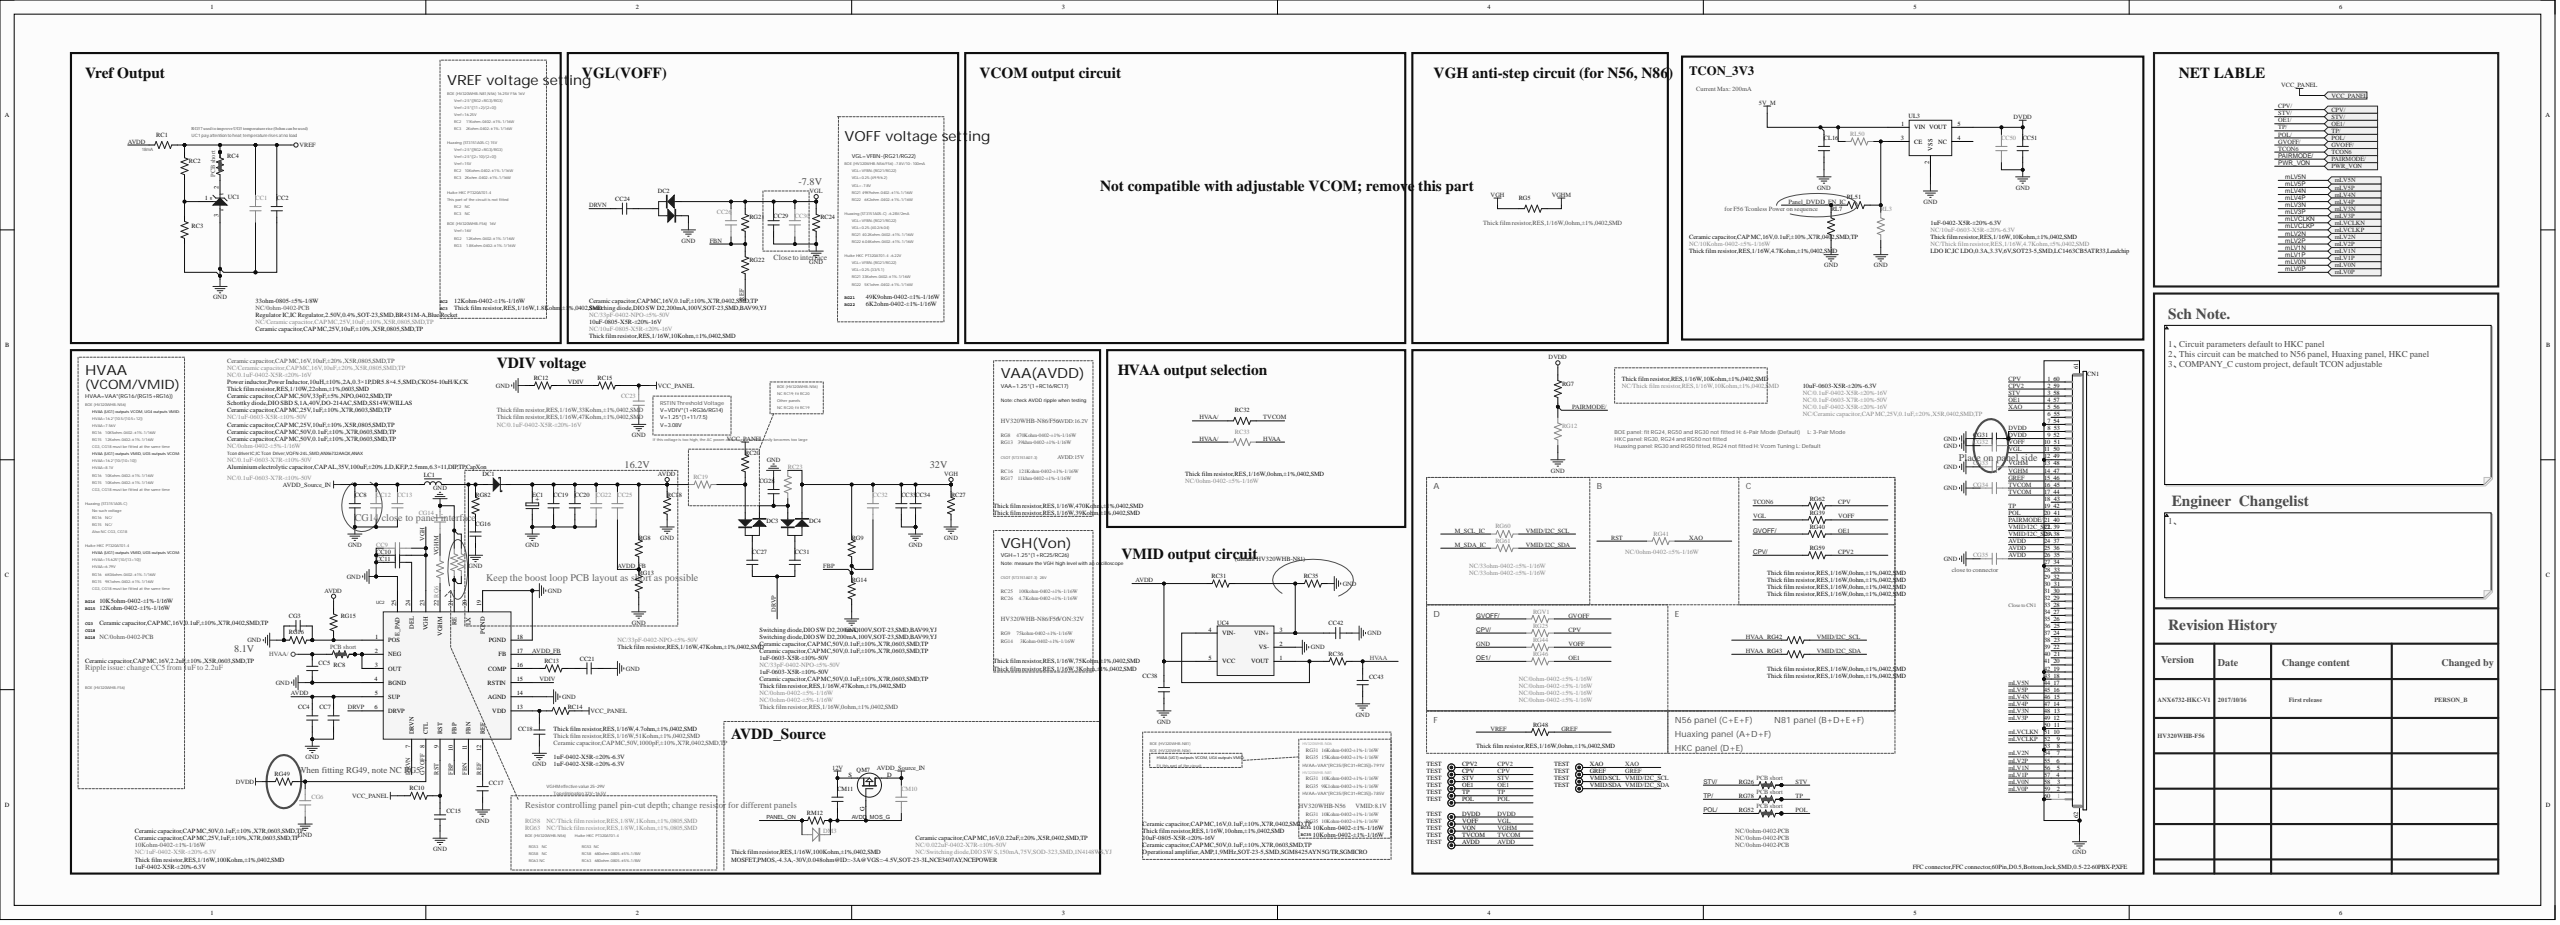Circuit board | Altium Designer | 719 parts | 352 nets | one sheet of the schematic
Parts on this sheet (reference | value | footprint):
AVDD | TEST | TP
CC1 | NC/Ceramic capacitor,CAP MC,25V,10uF,±10%,X5R,0805,SMD,TP | C0805
CC2 | Ceramic capacitor,CAP MC,25V,10uF,±10%,X5R,0805,SMD,TP | C0805
CC4 | Ceramic capacitor,CAP MC,25V,1uF,±10%,X7R,0603,SMD,TP | C0603
CC5 | Ceramic capacitor,CAP MC,16V,2.2uF,±10%,X5R,0603,SMD,TP | C0603
CC7 | Ceramic capacitor,CAP MC,50V,0.1uF,±10%,X7R,0603,SMD,TP | C0603
CC8 | Ceramic capacitor,CAP MC,16V,10uF,±20%,X5R,0805,SMD,TP | C0805
CC9 | NC/0.1uF-0603-X7R-±10%-50V | C0603
CC10 | Ceramic capacitor,CAP MC,50V,0.1uF,±10%,X7R,0603,SMD,TP | C0603
CC11 | Ceramic capacitor,CAP MC,50V,0.1uF,±10%,X7R,0603,SMD,TP | C0603
CC12 | NC/Ceramic capacitor,CAP MC,16V,10uF,±20%,X5R,0805,SMD,TP | C0805
CC13 | NC/0.1uF-0402-X5R-±20%-16V | C0402
CC15 | 1uF-0402-X5R-±20%-6.3V | C0402
CC17 | 1uF-0402-X5R-±20%-6.3V | C0402
CC18 | 1uF-0402-X5R-±20%-6.3V | C0402
CC19 | Ceramic capacitor,CAP MC,25V,10uF,±10%,X5R,0805,SMD,TP | C0805
CC20 | Ceramic capacitor,CAP MC,25V,1uF,±10%,X7R,0603,SMD,TP | C0603
CC21 | Ceramic capacitor,CAP MC,50V,1000pF,±10%,X7R,0402,SMD,TP | C0402
CC23 | NC/0.1uF-0402-X5R-±20%-16V | C0402
CC24 | Ceramic capacitor,CAP MC,16V,0.1uF,±10%,X7R,0402,SMD,TP | C0402
CC25 | NC/33pF-0402-NPO-±5%-50V | C0402
CC26 | NC/33pF-0402-NPO-±5%-50V | C0402
CC27 | Ceramic capacitor,CAP MC,50V,0.1uF,±10%,X7R,0603,SMD,TP | C0603
CC29 | 10uF-0805-X5R-±20%-16V | C0805
CC30 | NC/10uF-0805-X5R-±20%-16V | C0805
CC31 | Ceramic capacitor,CAP MC,50V,0.1uF,±10%,X7R,0603,SMD,TP | C0603
CC32 | NC/33pF-0402-NPO-±5%-50V | C0402
CC33 | 1uF-0603-X5R-±10%-50V | C0603
CC34 | Ceramic capacitor,CAP MC,50V,0.1uF,±10%,X7R,0603,SMD,TP | C0603
CC38 | Ceramic capacitor,CAP MC,50V,0.1uF,±10%,X7R,0603,SMD,TP | C0603
CC42 | Ceramic capacitor,CAP MC,16V,0.1uF,±10%,X7R,0402,SMD,TP | C0402
CC43 | 10uF-0805-X5R-±20%-16V | C0805
CC50 | NC/10uF-0603-X5R-±20%-6.3V | C0603
CC51 | 1uF-0402-X5R-±20%-6.3V | C0402
CG3 | Ceramic capacitor,CAP MC,16V,0.1uF,±10%,X7R,0402,SMD,TP | C0402
CG6 | NC/1uF-0402-X5R-±20%-6.3V | C0402
CG14 | NC/0.1uF-0603-X7R-±10%-50V | C0603
CG16 | Ceramic capacitor,CAP MC,50V,33pF,±5%,NPO,0402,SMD,TP | C0402
CG22 | NC/1uF-0603-X5R-±10%-50V | C0603
CG28 | 1uF-0603-X5R-±10%-50V | C0603
CG31 | 10uF-0603-X5R-±20%-6.3V | C0603
CG32 | NC/0.1uF-0402-X5R-±20%-16V | C0402
CG33 | NC/0.1uF-0603-X7R-±10%-50V | C0603
CG34 | NC/0.1uF-0402-X5R-±20%-16V | C0402
CG35 | NC/Ceramic capacitor,CAP MC,25V,0.1uF,±20%,X5R,0402,SMD,TP | C0402
CL16 | Ceramic capacitor,CAP MC,16V,0.1uF,±10%,X7R,0402,SMD,TP | C0402
CM10 | NC/0.022uF-0402-X7R-±10%-50V | C0402
CM11 | Ceramic capacitor,CAP MC,16V,0.22uF,±20%,X5R,0402,SMD,TP | C0402
CN1 | FFC connector,FFC connector,60Pin,D0.5,Bottom,lock,SMD,0.5-22-60PBX-P,XFE | FFC60H/0.5S-11
CPV | TEST | TP
CPV2 | TEST | TP
DC1 | Schottky diode,DIO SBD S,1A,40V,DO-214AC,SMD,SS14W,WILLAS | DIODE-S-1
DC2 | Switching diode,DIO SW D2,200mA,100V,SOT-23,SMD,BAV99,YJ | SO-23
DC3 | Switching diode,DIO SW D2,200mA,100V,SOT-23,SMD,BAV99,YJ | SO-23
DC4 | Switching diode,DIO SW D2,200mA,100V,SOT-23,SMD,BAV99,YJ | SO-23
DM3 | NC/Switching diode,DIO SW S,150mA,75V,SOD-323,SMD,1N4148WS,YJ | DIODE-S-12
DVDD | TEST | TP
GREF | TEST | TP
LC1 | Power inductor,Power Inductor,10uH,±10%,2A,0.3×1P,DR5.8×4.5,SMD,CKO54-10uH/K,CK | L(5.8*4.5)-S
OE1 | TEST | TP
POL | TEST | TP
QM7 | MOSFET,PMOS,-4.3A,-30V,0.048ohm@ID=-3A@VGS=-4.5V,SOT-23-3L,NCE3407AY,NCEPOWER | SOT-23-1
RC1 | 33ohm-0805-±5%-1/8W | R0805
RC2 | 12Kohm-0402-±1%-1/16W | R0402
RC3 | Thick film resistor,RES,1/16W,1.8Kohm,±1%,0402,SMD | R0402
RC4 | NC/0ohm-0402-PCB | R0402SC
RC8 | NC/0ohm-0402-PCB | R0402SC
RC10 | Thick film resistor,RES,1/16W,100Kohm,±1%,0402,SMD | R0402
RC12 | Thick film resistor,RES,1/16W,33Kohm,±1%,0402,SMD | R0402
RC13 | Thick film resistor,RES,1/16W,51Kohm,±1%,0402,SMD | R0402
RC14 | Thick film resistor,RES,1/16W,4.7ohm,±1%,0402,SMD | R0402
RC15 | Thick film resistor,RES,1/16W,47Kohm,±1%,0402,SMD | R0402
RC18 | Thick film resistor,RES,1/16W,47Kohm,±1%,0402,SMD | R0402
RC19 | NC/0ohm-0402-±5%-1/16W | R0402
RC20 | Thick film resistor,RES,1/16W,0ohm,±1%,0402,SMD | R0402
RC23 | NC/0ohm-0402-±5%-1/16W | R0402
RC24 | Thick film resistor,RES,1/16W,10Kohm,±1%,0402,SMD | R0402
RC27 | Thick film resistor,RES,1/16W,47Kohm,±1%,0402,SMD | R0402
RC31 | 10Kohm-0402-±1%-1/16W | R0402
RC32 | Thick film resistor,RES,1/16W,0ohm,±1%,0402,SMD | R0402
RC33 | NC/0ohm-0402-±5%-1/16W | R0402
RC35 | 10Kohm-0402-±1%-1/16W | R0402
RC36 | Thick film resistor,RES,1/16W,10ohm,±1%,0402,SMD | R0402
RG5 | Thick film resistor,RES,1/16W,0ohm,±1%,0402,SMD | R0402
RG6 | NC/0ohm-0402-±5%-1/16W | R0402
RG7 | Thick film resistor,RES,1/16W,10Kohm,±1%,0402,SMD | R0402
RG8 | Thick film resistor,RES,1/16W,470Kohm,±1%,0402,SMD | R0402
RG9 | Thick film resistor,RES,1/16W,75Kohm,±1%,0402,SMD | R0402
RG12 | NC/Thick film resistor,RES,1/16W,10Kohm,±1%,0402,SMD | R0402
RG13 | Thick film resistor,RES,1/16W,39Kohm,±1%,0402,SMD | R0402
RG14 | Thick film resistor,RES,1/16W,3Kohm,±1%,0402,SMD | R0402
RG15 | 12Kohm-0402-±1%-1/16W | R0402
RG16 | 10K5ohm-0402-±1%-1/16W | R0402
RG21 | 49K9ohm-0402-±1%-1/16W | R0402
RG22 | 6K2ohm-0402-±1%-1/16W | R0402
RG25 | NC/0ohm-0402-±5%-1/16W | R0402
RG26 | NC/0ohm-0402-PCB | R0402SC
RG39 | Thick film resistor,RES,1/16W,0ohm,±1%,0402,SMD | R0402
RG40 | Thick film resistor,RES,1/16W,0ohm,±1%,0402,SMD | R0402
RG41 | NC/0ohm-0402-±5%-1/16W | R0402
RG42 | Thick film resistor,RES,1/16W,0ohm,±1%,0402,SMD | R0402
RG43 | Thick film resistor,RES,1/16W,0ohm,±1%,0402,SMD | R0402
RG44 | NC/0ohm-0402-±5%-1/16W | R0402
RG46 | NC/0ohm-0402-±5%-1/16W | R0402
RG48 | Thick film resistor,RES,1/16W,0ohm,±1%,0402,SMD | R0402
RG49 | 10Kohm-0402-±1%-1/16W | R0402
RG52 | NC/0ohm-0402-PCB | R0402SC
RG58 | NC/Thick film resistor,RES,1/8W,1Kohm,±1%,0805,SMD | R0805
RG59 | Thick film resistor,RES,1/16W,0ohm,±1%,0402,SMD | R0402
RG60 | NC/33ohm-0402-±5%-1/16W | R0402
RG61 | NC/33ohm-0402-±5%-1/16W | R0402
RG62 | Thick film resistor,RES,1/16W,0ohm,±1%,0402,SMD | R0402
RG63 | NC/Thick film resistor,RES,1/8W,1Kohm,±1%,0805,SMD | R0805
RG78 | NC/0ohm-0402-PCB | R0402SC
RG82 | Thick film resistor,RES,1/10W,22ohm,±1%,0603,SMD | R0603
RGV1 | NC/0ohm-0402-±5%-1/16W | R0402
RL3 | NC/Thick film resistor,RES,1/16W,4.7Kohm,±5%,0402,SMD | R0402
RL7 | Thick film resistor,RES,1/16W,4.7Kohm,±1%,0402,SMD | R0402
RL50 | NC/10Kohm-0402-±5%-1/16W | R0402
RL51 | Thick film resistor,RES,1/16W,10Kohm,±1%,0402,SMD | R0402
RM12 | Thick film resistor,RES,1/16W,100Kohm,±1%,0402,SMD | R0402
STV | TEST | TP
TVCOM | TEST | TP
UC1 | Regulator IC,IC Regulator,2.50V,0.4%,SOT-23,SMD,BR431M-A,Blue Rocket | SO-23-1
UC2 | Tcon driver IC,IC Tcon  Driver,VQFN-24L,SMD,ANX6732AAQX,ANAX | QFN24/0.5-5
UC4 | Operational amplifier,AMP,1,9MHz,SOT-23-5,SMD,SGM8425AYN5G/TR,SGMICRO | SOT-23-5
UL3 | LDO IC,IC LDO,0.3A,3.3V,6V,SOT23-5,SMD,LC1463CB5ATR33,Leadchip | SOP23-5-1
VMID/SCL | TEST | TP
VMID/SDA | TEST | TP
VOFF | TEST | TP
VON | TEST | TP
XAO | TEST | TP
Nets of these parts (net: part-pin ...):
XAO: RG41-2 XAO-1 CN1-56
VREF: CC1-2 CC2-2 RC1-2 RC2-2 RC4-2 RC4-3 RG48-1
VOFF: CG32-2 RG39-2 RG44-2 CN1-51
VMID/I2C_SDA: RG43-2 RG61-2 VMID/SDA-1 CN1-38
VMID/I2C_SCL: RG42-2 RG60-2 VMID/SCL-1 CN1-39
VGL: CC26-2 CC29-1 CC30-1 DC2-1 RC24-2 RG21-2 RG39-1 VOFF-1 CN1-50
VGHM: CG14-1 CG33-2 RG5-1 RG6-2 VON-1 CN1-47 CN1-48
VGH: CC9-1 CC10-1 CC32-2 CC33-2 CC34-2 DC4-3 RC23-2 RC27-2 RG5-2 RG9-2 UC2-23
VDIV: RC12-2 RC15-1 UC2-15
VCC_PANEL: CC23-2 RC10-2 RC14-2 RC15-2 RC20-1
TVCOM: CG34-2 RC32-1 TVCOM-1 CN1-44 CN1-45
TP/: RG78-1
TP: RG78-2 RG78-3 CN1-42
TCON6: RG62-1
STV/: RG26-1
STV: RG26-2 RG26-3 STV-1 CN1-58
RST: CC15-1 RC10-1 RG41-1 UC2-9
REF: CC17-2 RG22-1 UC2-12
POL/: RG52-1
POL: POL-1 RG52-2 RG52-3 CN1-41
PANEL_ON: DM3-A RM12-1
Panel_DVDD_EN_IC: RL7-2 RL51-1
PAIRMODE/: RG7-1 RG12-2 CN1-40
OE1/: RG46-1
OE1: OE1-1 RG40-2 RG46-2 CN1-57
NetRL3_2: RL3-2 RL50-2 RL51-2 UL3-3
NetRG58_1: RG58-1 RG63-1 UC2-21
NetRG6_1: RG6-1 UC2-22
NetRC36_1: RC36-1 UC4-1 UC4-4
NetRC13_1: RC13-1 UC2-16
NetRC8_2: RC8-2 RC8-3 UC2-2 UC2-3
NetRC4_1: RC4-1 UC1-2
NetRC2_1: RC2-1 RC3-2 UC1-1
NetDC3_1: DC3-1 RC19-1 RC20-2
NetDC1_A: DC1-A LC1-2 RG82-2 UC2-20
NetCG28_1: CG28-1 DC3-3 DC4-1 RC23-1
NetCG16_2: CG16-2 RG82-1
NetCG3_1: CG3-1 RG15-1 RG16-2 UC2-1
NetCC42_1: CC42-1 RC31-2 RC35-1 UC4-3
NetCC31_1: CC31-1 DC4-2
NetCC27_1: CC27-1 DC3-2
NetCC24_2: CC24-2 DC2-2
NetCC21_1: CC21-1 RC13-2
NetCC18_2: CC18-2 RC14-1 UC2-13
NetCC11_1: CC11-1 UC2-24
mLVCLKP: CN1-9
mLVCLKN: CN1-10
mLV5P: CN1-16
mLV5N: CN1-17
mLV4P: CN1-14
mLV4N: CN1-15
mLV3P: CN1-12
mLV3N: CN1-13
mLV2P: CN1-6
mLV2N: CN1-7
mLV1P: CN1-4
mLV1N: CN1-5
mLV0P: CN1-2
mLV0N: CN1-3
M_SDA_IC: RG61-1
M_SCL_IC: RG60-1
HVAA/: CC5-1 RC8-1 RC32-2 RC33-1
HVAA: CC43-2 RC33-2 RC36-2 RG42-1 RG43-1
GVOFF/: RG40-1 RGV1-1
GVOFF: CG6-1 RG49-1 RGV1-2 UC2-8
GREF: GREF-1 RG48-2 CN1-46
GND: CC1-1 CC2-1 CC4-2 CC5-2 CC7-1 CC8-1 CC9-2 CC10-2 CC11-2 CC12-1 CC13-1 CC15-2 CC17-1 CC18-1 CC19-2 CC20-2 CC21-2 CC23-1 CC29-2 CC30-2 CC33-1 CC34-1 CC38-1 CC42-2 CC43-1 CC50-2 CC51-1 CG3-2 CG6-2 CG14-2 CG16-1 CG22-2 CG28-2 CG31-1 CG32-1 CG33-1 CG34-1 CG35-2 CL16-2 DC2-3 RC3-1 RC12-1 RC18-1 RC24-1 RC27-1 RC35-2 RG12-1 RG13-1 RG14-1 RG16-1 RG44-1 RG58-2 RG63-2 RL3-1 RL7-1 UC1-3 UC4-2 UL3-2 CN1-1 CN1-8 CN1-11 CN1-18 CN1-19 CN1-34 CN1-49 CN1-54 CN1-61 CN1-62 UC2-4 UC2-14 UC2-18 UC2-19 UC2-25
FBP: CC32-1 RG9-1 RG14-2 UC2-10
FBN: CC26-1 RG21-1 RG22-2 UC2-11
DVDD: CC50-1 CC51-2 CG31-2 DVDD-1 RG7-2 RG49-2 UL3-5 CN1-52 CN1-53
DRVP: CC27-2 CC31-2 UC2-6
DRVN: CC24-1 UC2-7
CPV/: RG25-1 RG59-1
CPV2: CPV2-1 RG59-2 CN1-59
CPV: CPV-1 RG25-2 RG62-2 CN1-60
AVDD_Source_IN: CC8-2 CC12-2 CC13-2 CM10-1 LC1-1 QM7-D
AVDD_MOS_G: CM10-2 CM11-1 DM3-K QM7-G RM12-2
AVDD_FB: CC25-1 RG8-1 RG13-2 UC2-17
AVDD: AVDD-1 CC4-1 CC7-2 CC19-1 CC20-1 CC25-2 CC38-2 CG22-1 CG35-1 DC1-K RC1-1 RC18-2 RC19-2 RC31-1 RG8-2 RG15-2 UC4-5 CN1-35 CN1-36 CN1-37 UC2-5
12V: CM11-2 QM7-S
5V_M: CL16-1 RL50-1 UL3-1